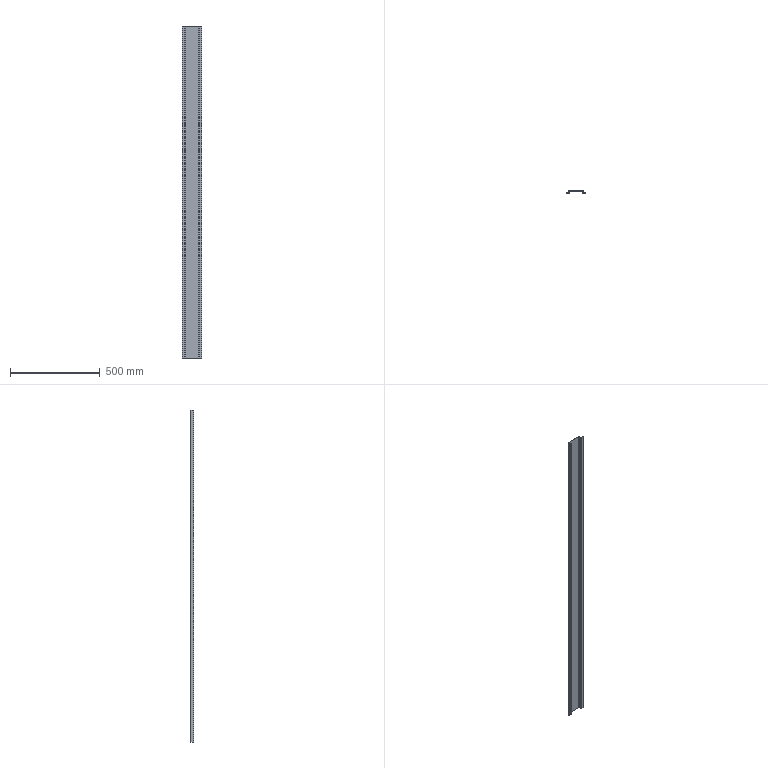Part | SolidWorks | features FlatPattern 1, SMBaseFlange 1, SheetMetal 1 | 1 solid | 38 faces | box 110 x 17 x 1845 mm | volume 384278 mm3 | plane 30 | cylinder 8 | commonest cylinder face diameters 1 x4 4 x4
STEP:
#1=CARTESIAN_POINT('',(-40.,0.5,922.5));
#2=VERTEX_POINT('',#1);
#3=CARTESIAN_POINT('',(-38.5,0.5,922.5));
#4=VERTEX_POINT('',#3);
#5=CARTESIAN_POINT('',(-40.,0.5,922.5));
#6=DIRECTION('',(1.,0.,0.));
#7=VECTOR('',#6,1000.);
#8=LINE('',#5,#7);
#9=EDGE_CURVE('',#2,#4,#8,.T.);
#10=ORIENTED_EDGE('',*,*,#9,.F.);
#11=CARTESIAN_POINT('',(-40.5,0.,922.5));
#12=VERTEX_POINT('',#11);
#13=CARTESIAN_POINT('',(-40.5,0.5,922.5));
#14=DIRECTION('',(0.,0.,-1.));
#15=DIRECTION('',(-1.,0.,0.));
#16=AXIS2_PLACEMENT_3D('',#13,#14,#15);
#17=CIRCLE('',#16,0.5);
#18=EDGE_CURVE('',#2,#12,#17,.T.);
#19=ORIENTED_EDGE('',*,*,#18,.T.);
#20=CARTESIAN_POINT('',(-40.5,-1.5,922.5));
#21=VERTEX_POINT('',#20);
#22=CARTESIAN_POINT('',(-40.5,-1.5,922.5));
#23=DIRECTION('',(0.,1.,0.));
#24=VECTOR('',#23,1000.);
#25=LINE('',#22,#24);
#26=EDGE_CURVE('',#21,#12,#25,.T.);
#27=ORIENTED_EDGE('',*,*,#26,.F.);
#28=CARTESIAN_POINT('',(-40.5,0.5,922.5));
#29=DIRECTION('',(0.,0.,-1.));
#30=DIRECTION('',(1.,0.,0.));
#31=AXIS2_PLACEMENT_3D('',#28,#29,#30);
#32=CIRCLE('',#31,2.);
#33=EDGE_CURVE('',#4,#21,#32,.T.);
#34=ORIENTED_EDGE('',*,*,#33,.F.);
#35=EDGE_LOOP('',(#10,#19,#27,#34));
#36=FACE_OUTER_BOUND('',#35,.T.);
#37=CARTESIAN_POINT('',(-40.,0.5,922.5));
#38=DIRECTION('',(0.,0.,1.));
#39=DIRECTION('',(1.,0.,0.));
#40=AXIS2_PLACEMENT_3D('',#37,#38,#39);
#41=PLANE('',#40);
#42=ADVANCED_FACE('',(#36),#41,.T.);
#43=CARTESIAN_POINT('',(-40.,13.5,922.5));
#44=VERTEX_POINT('',#43);
#45=CARTESIAN_POINT('',(-40.,0.,922.5));
#46=DIRECTION('',(0.,-1.,0.));
#47=VECTOR('',#46,1000.);
#48=LINE('',#45,#47);
#49=EDGE_CURVE('',#44,#2,#48,.T.);
#50=ORIENTED_EDGE('',*,*,#49,.T.);
#51=ORIENTED_EDGE('',*,*,#9,.T.);
#52=CARTESIAN_POINT('',(-38.5,13.5,922.5));
#53=VERTEX_POINT('',#52);
#54=CARTESIAN_POINT('',(-38.5,0.,922.5));
#55=DIRECTION('',(0.,-1.,0.));
#56=VECTOR('',#55,1000.);
#57=LINE('',#54,#56);
#58=EDGE_CURVE('',#53,#4,#57,.T.);
#59=ORIENTED_EDGE('',*,*,#58,.F.);
#60=CARTESIAN_POINT('',(-38.5,13.5,922.5));
#61=DIRECTION('',(-1.,0.,0.));
#62=VECTOR('',#61,1000.);
#63=LINE('',#60,#62);
#64=EDGE_CURVE('',#53,#44,#63,.T.);
#65=ORIENTED_EDGE('',*,*,#64,.T.);
#66=EDGE_LOOP('',(#50,#51,#59,#65));
#67=FACE_OUTER_BOUND('',#66,.T.);
#68=CARTESIAN_POINT('',(-40.5,-1.5,922.5));
#69=DIRECTION('',(0.,0.,1.));
#70=DIRECTION('',(1.,0.,0.));
#71=AXIS2_PLACEMENT_3D('',#68,#69,#70);
#72=PLANE('',#71);
#73=ADVANCED_FACE('',(#67),#72,.T.);
#74=CARTESIAN_POINT('',(-40.5,0.,-922.5));
#75=VERTEX_POINT('',#74);
#76=CARTESIAN_POINT('',(-40.5,-1.5,-922.5));
#77=VERTEX_POINT('',#76);
#78=CARTESIAN_POINT('',(-40.5,0.,-922.5));
#79=DIRECTION('',(0.,-1.,0.));
#80=VECTOR('',#79,1000.);
#81=LINE('',#78,#80);
#82=EDGE_CURVE('',#75,#77,#81,.T.);
#83=ORIENTED_EDGE('',*,*,#82,.F.);
#84=CARTESIAN_POINT('',(-40.,0.5,-922.5));
#85=VERTEX_POINT('',#84);
#86=CARTESIAN_POINT('',(-40.5,0.5,-922.5));
#87=DIRECTION('',(0.,0.,-1.));
#88=DIRECTION('',(-1.,0.,0.));
#89=AXIS2_PLACEMENT_3D('',#86,#87,#88);
#90=CIRCLE('',#89,0.5);
#91=EDGE_CURVE('',#85,#75,#90,.T.);
#92=ORIENTED_EDGE('',*,*,#91,.F.);
#93=CARTESIAN_POINT('',(-38.5,0.5,-922.5));
#94=VERTEX_POINT('',#93);
#95=CARTESIAN_POINT('',(-38.5,0.5,-922.5));
#96=DIRECTION('',(-1.,0.,0.));
#97=VECTOR('',#96,1000.);
#98=LINE('',#95,#97);
#99=EDGE_CURVE('',#94,#85,#98,.T.);
#100=ORIENTED_EDGE('',*,*,#99,.F.);
#101=CARTESIAN_POINT('',(-40.5,0.5,-922.5));
#102=DIRECTION('',(0.,0.,-1.));
#103=DIRECTION('',(1.,0.,0.));
#104=AXIS2_PLACEMENT_3D('',#101,#102,#103);
#105=CIRCLE('',#104,2.);
#106=EDGE_CURVE('',#94,#77,#105,.T.);
#107=ORIENTED_EDGE('',*,*,#106,.T.);
#108=EDGE_LOOP('',(#83,#92,#100,#107));
#109=FACE_OUTER_BOUND('',#108,.T.);
#110=CARTESIAN_POINT('',(-40.5,0.,-922.5));
#111=DIRECTION('',(0.,0.,-1.));
#112=DIRECTION('',(-1.,0.,0.));
#113=AXIS2_PLACEMENT_3D('',#110,#111,#112);
#114=PLANE('',#113);
#115=ADVANCED_FACE('',(#109),#114,.T.);
#116=CARTESIAN_POINT('',(-55.,0.,-922.5));
#117=VERTEX_POINT('',#116);
#118=CARTESIAN_POINT('',(-55.,0.,-922.5));
#119=DIRECTION('',(-1.,0.,0.));
#120=VECTOR('',#119,1000.);
#121=LINE('',#118,#120);
#122=EDGE_CURVE('',#75,#117,#121,.T.);
#123=ORIENTED_EDGE('',*,*,#122,.F.);
#124=ORIENTED_EDGE('',*,*,#82,.T.);
#125=CARTESIAN_POINT('',(-55.,-1.5,-922.5));
#126=VERTEX_POINT('',#125);
#127=CARTESIAN_POINT('',(-55.,-1.5,-922.5));
#128=DIRECTION('',(-1.,0.,0.));
#129=VECTOR('',#128,1000.);
#130=LINE('',#127,#129);
#131=EDGE_CURVE('',#77,#126,#130,.T.);
#132=ORIENTED_EDGE('',*,*,#131,.T.);
#133=CARTESIAN_POINT('',(-55.,-1.5,-922.5));
#134=DIRECTION('',(0.,1.,0.));
#135=VECTOR('',#134,1000.);
#136=LINE('',#133,#135);
#137=EDGE_CURVE('',#126,#117,#136,.T.);
#138=ORIENTED_EDGE('',*,*,#137,.T.);
#139=EDGE_LOOP('',(#123,#124,#132,#138));
#140=FACE_OUTER_BOUND('',#139,.T.);
#141=CARTESIAN_POINT('',(-38.5,0.5,-922.5));
#142=DIRECTION('',(0.,0.,-1.));
#143=DIRECTION('',(-1.,0.,0.));
#144=AXIS2_PLACEMENT_3D('',#141,#142,#143);
#145=PLANE('',#144);
#146=ADVANCED_FACE('',(#140),#145,.T.);
#147=CARTESIAN_POINT('',(-38.,15.5,922.5));
#148=VERTEX_POINT('',#147);
#149=CARTESIAN_POINT('',(-38.,14.,922.5));
#150=VERTEX_POINT('',#149);
#151=CARTESIAN_POINT('',(-38.,15.5,922.5));
#152=DIRECTION('',(0.,-1.,0.));
#153=VECTOR('',#152,1000.);
#154=LINE('',#151,#153);
#155=EDGE_CURVE('',#148,#150,#154,.T.);
#156=ORIENTED_EDGE('',*,*,#155,.F.);
#157=CARTESIAN_POINT('',(-38.,13.5,922.5));
#158=DIRECTION('',(0.,0.,1.));
#159=DIRECTION('',(1.,0.,0.));
#160=AXIS2_PLACEMENT_3D('',#157,#158,#159);
#161=CIRCLE('',#160,2.);
#162=EDGE_CURVE('',#148,#44,#161,.T.);
#163=ORIENTED_EDGE('',*,*,#162,.T.);
#164=ORIENTED_EDGE('',*,*,#64,.F.);
#165=CARTESIAN_POINT('',(-38.,13.5,922.5));
#166=DIRECTION('',(0.,0.,1.));
#167=DIRECTION('',(1.,0.,0.));
#168=AXIS2_PLACEMENT_3D('',#165,#166,#167);
#169=CIRCLE('',#168,0.5);
#170=EDGE_CURVE('',#150,#53,#169,.T.);
#171=ORIENTED_EDGE('',*,*,#170,.F.);
#172=EDGE_LOOP('',(#156,#163,#164,#171));
#173=FACE_OUTER_BOUND('',#172,.T.);
#174=CARTESIAN_POINT('',(-38.,15.5,922.5));
#175=DIRECTION('',(0.,0.,1.));
#176=DIRECTION('',(1.,0.,0.));
#177=AXIS2_PLACEMENT_3D('',#174,#175,#176);
#178=PLANE('',#177);
#179=ADVANCED_FACE('',(#173),#178,.T.);
#180=CARTESIAN_POINT('',(38.,15.5,922.5));
#181=VERTEX_POINT('',#180);
#182=CARTESIAN_POINT('',(-40.,15.5,922.5));
#183=DIRECTION('',(-1.,0.,0.));
#184=VECTOR('',#183,1000.);
#185=LINE('',#182,#184);
#186=EDGE_CURVE('',#181,#148,#185,.T.);
#187=ORIENTED_EDGE('',*,*,#186,.T.);
#188=ORIENTED_EDGE('',*,*,#155,.T.);
#189=CARTESIAN_POINT('',(38.,14.,922.5));
#190=VERTEX_POINT('',#189);
#191=CARTESIAN_POINT('',(-40.,14.,922.5));
#192=DIRECTION('',(-1.,0.,0.));
#193=VECTOR('',#192,1000.);
#194=LINE('',#191,#193);
#195=EDGE_CURVE('',#190,#150,#194,.T.);
#196=ORIENTED_EDGE('',*,*,#195,.F.);
#197=CARTESIAN_POINT('',(38.,14.,922.5));
#198=DIRECTION('',(0.,1.,0.));
#199=VECTOR('',#198,1000.);
#200=LINE('',#197,#199);
#201=EDGE_CURVE('',#190,#181,#200,.T.);
#202=ORIENTED_EDGE('',*,*,#201,.T.);
#203=EDGE_LOOP('',(#187,#188,#196,#202));
#204=FACE_OUTER_BOUND('',#203,.T.);
#205=CARTESIAN_POINT('',(-38.5,13.5,922.5));
#206=DIRECTION('',(0.,0.,1.));
#207=DIRECTION('',(1.,0.,0.));
#208=AXIS2_PLACEMENT_3D('',#205,#206,#207);
#209=PLANE('',#208);
#210=ADVANCED_FACE('',(#204),#209,.T.);
#211=CARTESIAN_POINT('',(-40.,13.5,-922.5));
#212=VERTEX_POINT('',#211);
#213=CARTESIAN_POINT('',(-38.5,13.5,-922.5));
#214=VERTEX_POINT('',#213);
#215=CARTESIAN_POINT('',(-40.,13.5,-922.5));
#216=DIRECTION('',(1.,0.,0.));
#217=VECTOR('',#216,1000.);
#218=LINE('',#215,#217);
#219=EDGE_CURVE('',#212,#214,#218,.T.);
#220=ORIENTED_EDGE('',*,*,#219,.F.);
#221=CARTESIAN_POINT('',(-38.,15.5,-922.5));
#222=VERTEX_POINT('',#221);
#223=CARTESIAN_POINT('',(-38.,13.5,-922.5));
#224=DIRECTION('',(0.,0.,1.));
#225=DIRECTION('',(1.,0.,0.));
#226=AXIS2_PLACEMENT_3D('',#223,#224,#225);
#227=CIRCLE('',#226,2.);
#228=EDGE_CURVE('',#222,#212,#227,.T.);
#229=ORIENTED_EDGE('',*,*,#228,.F.);
#230=CARTESIAN_POINT('',(-38.,14.,-922.5));
#231=VERTEX_POINT('',#230);
#232=CARTESIAN_POINT('',(-38.,14.,-922.5));
#233=DIRECTION('',(0.,1.,0.));
#234=VECTOR('',#233,1000.);
#235=LINE('',#232,#234);
#236=EDGE_CURVE('',#231,#222,#235,.T.);
#237=ORIENTED_EDGE('',*,*,#236,.F.);
#238=CARTESIAN_POINT('',(-38.,13.5,-922.5));
#239=DIRECTION('',(0.,0.,1.));
#240=DIRECTION('',(1.,0.,0.));
#241=AXIS2_PLACEMENT_3D('',#238,#239,#240);
#242=CIRCLE('',#241,0.5);
#243=EDGE_CURVE('',#231,#214,#242,.T.);
#244=ORIENTED_EDGE('',*,*,#243,.T.);
#245=EDGE_LOOP('',(#220,#229,#237,#244));
#246=FACE_OUTER_BOUND('',#245,.T.);
#247=CARTESIAN_POINT('',(-40.,13.5,-922.5));
#248=DIRECTION('',(0.,0.,-1.));
#249=DIRECTION('',(-1.,0.,0.));
#250=AXIS2_PLACEMENT_3D('',#247,#248,#249);
#251=PLANE('',#250);
#252=ADVANCED_FACE('',(#246),#251,.T.);
#253=CARTESIAN_POINT('',(-40.,0.,-922.5));
#254=DIRECTION('',(0.,-1.,0.));
#255=VECTOR('',#254,1000.);
#256=LINE('',#253,#255);
#257=EDGE_CURVE('',#212,#85,#256,.T.);
#258=ORIENTED_EDGE('',*,*,#257,.F.);
#259=ORIENTED_EDGE('',*,*,#219,.T.);
#260=CARTESIAN_POINT('',(-38.5,0.,-922.5));
#261=DIRECTION('',(0.,-1.,0.));
#262=VECTOR('',#261,1000.);
#263=LINE('',#260,#262);
#264=EDGE_CURVE('',#214,#94,#263,.T.);
#265=ORIENTED_EDGE('',*,*,#264,.T.);
#266=ORIENTED_EDGE('',*,*,#99,.T.);
#267=EDGE_LOOP('',(#258,#259,#265,#266));
#268=FACE_OUTER_BOUND('',#267,.T.);
#269=CARTESIAN_POINT('',(-38.,14.,-922.5));
#270=DIRECTION('',(0.,0.,-1.));
#271=DIRECTION('',(-1.,0.,0.));
#272=AXIS2_PLACEMENT_3D('',#269,#270,#271);
#273=PLANE('',#272);
#274=ADVANCED_FACE('',(#268),#273,.T.);
#275=CARTESIAN_POINT('',(40.,13.5,922.5));
#276=VERTEX_POINT('',#275);
#277=CARTESIAN_POINT('',(38.5,13.5,922.5));
#278=VERTEX_POINT('',#277);
#279=CARTESIAN_POINT('',(40.,13.5,922.5));
#280=DIRECTION('',(-1.,0.,0.));
#281=VECTOR('',#280,1000.);
#282=LINE('',#279,#281);
#283=EDGE_CURVE('',#276,#278,#282,.T.);
#284=ORIENTED_EDGE('',*,*,#283,.F.);
#285=CARTESIAN_POINT('',(38.,13.5,922.5));
#286=DIRECTION('',(0.,0.,1.));
#287=DIRECTION('',(1.,0.,0.));
#288=AXIS2_PLACEMENT_3D('',#285,#286,#287);
#289=CIRCLE('',#288,2.);
#290=EDGE_CURVE('',#276,#181,#289,.T.);
#291=ORIENTED_EDGE('',*,*,#290,.T.);
#292=ORIENTED_EDGE('',*,*,#201,.F.);
#293=CARTESIAN_POINT('',(38.,13.5,922.5));
#294=DIRECTION('',(0.,0.,1.));
#295=DIRECTION('',(1.,0.,0.));
#296=AXIS2_PLACEMENT_3D('',#293,#294,#295);
#297=CIRCLE('',#296,0.5);
#298=EDGE_CURVE('',#278,#190,#297,.T.);
#299=ORIENTED_EDGE('',*,*,#298,.F.);
#300=EDGE_LOOP('',(#284,#291,#292,#299));
#301=FACE_OUTER_BOUND('',#300,.T.);
#302=CARTESIAN_POINT('',(40.,13.5,922.5));
#303=DIRECTION('',(0.,0.,1.));
#304=DIRECTION('',(1.,0.,0.));
#305=AXIS2_PLACEMENT_3D('',#302,#303,#304);
#306=PLANE('',#305);
#307=ADVANCED_FACE('',(#301),#306,.T.);
#308=CARTESIAN_POINT('',(40.,0.5,922.5));
#309=VERTEX_POINT('',#308);
#310=CARTESIAN_POINT('',(40.,0.,922.5));
#311=DIRECTION('',(0.,1.,0.));
#312=VECTOR('',#311,1000.);
#313=LINE('',#310,#312);
#314=EDGE_CURVE('',#309,#276,#313,.T.);
#315=ORIENTED_EDGE('',*,*,#314,.T.);
#316=ORIENTED_EDGE('',*,*,#283,.T.);
#317=CARTESIAN_POINT('',(38.5,0.5,922.5));
#318=VERTEX_POINT('',#317);
#319=CARTESIAN_POINT('',(38.5,0.,922.5));
#320=DIRECTION('',(0.,1.,0.));
#321=VECTOR('',#320,1000.);
#322=LINE('',#319,#321);
#323=EDGE_CURVE('',#318,#278,#322,.T.);
#324=ORIENTED_EDGE('',*,*,#323,.F.);
#325=CARTESIAN_POINT('',(38.5,0.5,922.5));
#326=DIRECTION('',(1.,0.,0.));
#327=VECTOR('',#326,1000.);
#328=LINE('',#325,#327);
#329=EDGE_CURVE('',#318,#309,#328,.T.);
#330=ORIENTED_EDGE('',*,*,#329,.T.);
#331=EDGE_LOOP('',(#315,#316,#324,#330));
#332=FACE_OUTER_BOUND('',#331,.T.);
#333=CARTESIAN_POINT('',(38.,14.,922.5));
#334=DIRECTION('',(0.,0.,1.));
#335=DIRECTION('',(1.,0.,0.));
#336=AXIS2_PLACEMENT_3D('',#333,#334,#335);
#337=PLANE('',#336);
#338=ADVANCED_FACE('',(#332),#337,.T.);
#339=CARTESIAN_POINT('',(38.,15.5,-922.5));
#340=VERTEX_POINT('',#339);
#341=CARTESIAN_POINT('',(38.,14.,-922.5));
#342=VERTEX_POINT('',#341);
#343=CARTESIAN_POINT('',(38.,15.5,-922.5));
#344=DIRECTION('',(0.,-1.,0.));
#345=VECTOR('',#344,1000.);
#346=LINE('',#343,#345);
#347=EDGE_CURVE('',#340,#342,#346,.T.);
#348=ORIENTED_EDGE('',*,*,#347,.F.);
#349=CARTESIAN_POINT('',(40.,13.5,-922.5));
#350=VERTEX_POINT('',#349);
#351=CARTESIAN_POINT('',(38.,13.5,-922.5));
#352=DIRECTION('',(0.,0.,1.));
#353=DIRECTION('',(1.,0.,0.));
#354=AXIS2_PLACEMENT_3D('',#351,#352,#353);
#355=CIRCLE('',#354,2.);
#356=EDGE_CURVE('',#350,#340,#355,.T.);
#357=ORIENTED_EDGE('',*,*,#356,.F.);
#358=CARTESIAN_POINT('',(38.5,13.5,-922.5));
#359=VERTEX_POINT('',#358);
#360=CARTESIAN_POINT('',(38.5,13.5,-922.5));
#361=DIRECTION('',(1.,0.,0.));
#362=VECTOR('',#361,1000.);
#363=LINE('',#360,#362);
#364=EDGE_CURVE('',#359,#350,#363,.T.);
#365=ORIENTED_EDGE('',*,*,#364,.F.);
#366=CARTESIAN_POINT('',(38.,13.5,-922.5));
#367=DIRECTION('',(0.,0.,1.));
#368=DIRECTION('',(1.,0.,0.));
#369=AXIS2_PLACEMENT_3D('',#366,#367,#368);
#370=CIRCLE('',#369,0.5);
#371=EDGE_CURVE('',#359,#342,#370,.T.);
#372=ORIENTED_EDGE('',*,*,#371,.T.);
#373=EDGE_LOOP('',(#348,#357,#365,#372));
#374=FACE_OUTER_BOUND('',#373,.T.);
#375=CARTESIAN_POINT('',(38.,15.5,-922.5));
#376=DIRECTION('',(0.,0.,-1.));
#377=DIRECTION('',(-1.,0.,0.));
#378=AXIS2_PLACEMENT_3D('',#375,#376,#377);
#379=PLANE('',#378);
#380=ADVANCED_FACE('',(#374),#379,.T.);
#381=CARTESIAN_POINT('',(-40.,15.5,-922.5));
#382=DIRECTION('',(-1.,0.,0.));
#383=VECTOR('',#382,1000.);
#384=LINE('',#381,#383);
#385=EDGE_CURVE('',#340,#222,#384,.T.);
#386=ORIENTED_EDGE('',*,*,#385,.F.);
#387=ORIENTED_EDGE('',*,*,#347,.T.);
#388=CARTESIAN_POINT('',(-40.,14.,-922.5));
#389=DIRECTION('',(-1.,0.,0.));
#390=VECTOR('',#389,1000.);
#391=LINE('',#388,#390);
#392=EDGE_CURVE('',#342,#231,#391,.T.);
#393=ORIENTED_EDGE('',*,*,#392,.T.);
#394=ORIENTED_EDGE('',*,*,#236,.T.);
#395=EDGE_LOOP('',(#386,#387,#393,#394));
#396=FACE_OUTER_BOUND('',#395,.T.);
#397=CARTESIAN_POINT('',(38.5,13.5,-922.5));
#398=DIRECTION('',(0.,0.,-1.));
#399=DIRECTION('',(-1.,0.,0.));
#400=AXIS2_PLACEMENT_3D('',#397,#398,#399);
#401=PLANE('',#400);
#402=ADVANCED_FACE('',(#396),#401,.T.);
#403=CARTESIAN_POINT('',(40.5,0.,922.5));
#404=VERTEX_POINT('',#403);
#405=CARTESIAN_POINT('',(40.5,-1.5,922.5));
#406=VERTEX_POINT('',#405);
#407=CARTESIAN_POINT('',(40.5,0.,922.5));
#408=DIRECTION('',(0.,-1.,0.));
#409=VECTOR('',#408,1000.);
#410=LINE('',#407,#409);
#411=EDGE_CURVE('',#404,#406,#410,.T.);
#412=ORIENTED_EDGE('',*,*,#411,.F.);
#413=CARTESIAN_POINT('',(40.5,0.5,922.5));
#414=DIRECTION('',(0.,0.,-1.));
#415=DIRECTION('',(-1.,0.,0.));
#416=AXIS2_PLACEMENT_3D('',#413,#414,#415);
#417=CIRCLE('',#416,0.5);
#418=EDGE_CURVE('',#404,#309,#417,.T.);
#419=ORIENTED_EDGE('',*,*,#418,.T.);
#420=ORIENTED_EDGE('',*,*,#329,.F.);
#421=CARTESIAN_POINT('',(40.5,0.5,922.5));
#422=DIRECTION('',(0.,0.,-1.));
#423=DIRECTION('',(1.,0.,0.));
#424=AXIS2_PLACEMENT_3D('',#421,#422,#423);
#425=CIRCLE('',#424,2.);
#426=EDGE_CURVE('',#406,#318,#425,.T.);
#427=ORIENTED_EDGE('',*,*,#426,.F.);
#428=EDGE_LOOP('',(#412,#419,#420,#427));
#429=FACE_OUTER_BOUND('',#428,.T.);
#430=CARTESIAN_POINT('',(40.5,0.,922.5));
#431=DIRECTION('',(0.,0.,1.));
#432=DIRECTION('',(1.,0.,0.));
#433=AXIS2_PLACEMENT_3D('',#430,#431,#432);
#434=PLANE('',#433);
#435=ADVANCED_FACE('',(#429),#434,.T.);
#436=CARTESIAN_POINT('',(55.,0.,922.5));
#437=VERTEX_POINT('',#436);
#438=CARTESIAN_POINT('',(55.,0.,922.5));
#439=DIRECTION('',(-1.,0.,0.));
#440=VECTOR('',#439,1000.);
#441=LINE('',#438,#440);
#442=EDGE_CURVE('',#437,#404,#441,.T.);
#443=ORIENTED_EDGE('',*,*,#442,.T.);
#444=ORIENTED_EDGE('',*,*,#411,.T.);
#445=CARTESIAN_POINT('',(55.,-1.5,922.5));
#446=VERTEX_POINT('',#445);
#447=CARTESIAN_POINT('',(55.,-1.5,922.5));
#448=DIRECTION('',(-1.,0.,0.));
#449=VECTOR('',#448,1000.);
#450=LINE('',#447,#449);
#451=EDGE_CURVE('',#446,#406,#450,.T.);
#452=ORIENTED_EDGE('',*,*,#451,.F.);
#453=CARTESIAN_POINT('',(55.,0.,922.5));
#454=DIRECTION('',(0.,-1.,0.));
#455=VECTOR('',#454,1000.);
#456=LINE('',#453,#455);
#457=EDGE_CURVE('',#437,#446,#456,.T.);
#458=ORIENTED_EDGE('',*,*,#457,.F.);
#459=EDGE_LOOP('',(#443,#444,#452,#458));
#460=FACE_OUTER_BOUND('',#459,.T.);
#461=CARTESIAN_POINT('',(38.5,0.5,922.5));
#462=DIRECTION('',(0.,0.,1.));
#463=DIRECTION('',(1.,0.,0.));
#464=AXIS2_PLACEMENT_3D('',#461,#462,#463);
#465=PLANE('',#464);
#466=ADVANCED_FACE('',(#460),#465,.T.);
#467=CARTESIAN_POINT('',(40.,0.5,-922.5));
#468=VERTEX_POINT('',#467);
#469=CARTESIAN_POINT('',(38.5,0.5,-922.5));
#470=VERTEX_POINT('',#469);
#471=CARTESIAN_POINT('',(40.,0.5,-922.5));
#472=DIRECTION('',(-1.,0.,0.));
#473=VECTOR('',#472,1000.);
#474=LINE('',#471,#473);
#475=EDGE_CURVE('',#468,#470,#474,.T.);
#476=ORIENTED_EDGE('',*,*,#475,.F.);
#477=CARTESIAN_POINT('',(40.5,0.,-922.5));
#478=VERTEX_POINT('',#477);
#479=CARTESIAN_POINT('',(40.5,0.5,-922.5));
#480=DIRECTION('',(0.,0.,-1.));
#481=DIRECTION('',(-1.,0.,0.));
#482=AXIS2_PLACEMENT_3D('',#479,#480,#481);
#483=CIRCLE('',#482,0.5);
#484=EDGE_CURVE('',#478,#468,#483,.T.);
#485=ORIENTED_EDGE('',*,*,#484,.F.);
#486=CARTESIAN_POINT('',(40.5,-1.5,-922.5));
#487=VERTEX_POINT('',#486);
#488=CARTESIAN_POINT('',(40.5,-1.5,-922.5));
#489=DIRECTION('',(0.,1.,0.));
#490=VECTOR('',#489,1000.);
#491=LINE('',#488,#490);
#492=EDGE_CURVE('',#487,#478,#491,.T.);
#493=ORIENTED_EDGE('',*,*,#492,.F.);
#494=CARTESIAN_POINT('',(40.5,0.5,-922.5));
#495=DIRECTION('',(0.,0.,-1.));
#496=DIRECTION('',(1.,0.,0.));
#497=AXIS2_PLACEMENT_3D('',#494,#495,#496);
#498=CIRCLE('',#497,2.);
#499=EDGE_CURVE('',#487,#470,#498,.T.);
#500=ORIENTED_EDGE('',*,*,#499,.T.);
#501=EDGE_LOOP('',(#476,#485,#493,#500));
#502=FACE_OUTER_BOUND('',#501,.T.);
#503=CARTESIAN_POINT('',(40.,0.5,-922.5));
#504=DIRECTION('',(0.,0.,-1.));
#505=DIRECTION('',(-1.,0.,0.));
#506=AXIS2_PLACEMENT_3D('',#503,#504,#505);
#507=PLANE('',#506);
#508=ADVANCED_FACE('',(#502),#507,.T.);
#509=CARTESIAN_POINT('',(40.,0.,-922.5));
#510=DIRECTION('',(0.,1.,0.));
#511=VECTOR('',#510,1000.);
#512=LINE('',#509,#511);
#513=EDGE_CURVE('',#468,#350,#512,.T.);
#514=ORIENTED_EDGE('',*,*,#513,.F.);
#515=ORIENTED_EDGE('',*,*,#475,.T.);
#516=CARTESIAN_POINT('',(38.5,0.,-922.5));
#517=DIRECTION('',(0.,1.,0.));
#518=VECTOR('',#517,1000.);
#519=LINE('',#516,#518);
#520=EDGE_CURVE('',#470,#359,#519,.T.);
#521=ORIENTED_EDGE('',*,*,#520,.T.);
#522=ORIENTED_EDGE('',*,*,#364,.T.);
#523=EDGE_LOOP('',(#514,#515,#521,#522));
#524=FACE_OUTER_BOUND('',#523,.T.);
#525=CARTESIAN_POINT('',(40.5,-1.5,-922.5));
#526=DIRECTION('',(0.,0.,-1.));
#527=DIRECTION('',(-1.,0.,0.));
#528=AXIS2_PLACEMENT_3D('',#525,#526,#527);
#529=PLANE('',#528);
#530=ADVANCED_FACE('',(#524),#529,.T.);
#531=ORIENTED_EDGE('',*,*,#122,.T.);
#532=CARTESIAN_POINT('',(-55.,0.,922.5));
#533=VERTEX_POINT('',#532);
#534=CARTESIAN_POINT('',(-55.,0.,922.5));
#535=DIRECTION('',(0.,0.,-1.));
#536=VECTOR('',#535,1000.);
#537=LINE('',#534,#536);
#538=EDGE_CURVE('',#533,#117,#537,.T.);
#539=ORIENTED_EDGE('',*,*,#538,.F.);
#540=CARTESIAN_POINT('',(-55.,0.,922.5));
#541=DIRECTION('',(-1.,0.,0.));
#542=VECTOR('',#541,1000.);
#543=LINE('',#540,#542);
#544=EDGE_CURVE('',#12,#533,#543,.T.);
#545=ORIENTED_EDGE('',*,*,#544,.F.);
#546=CARTESIAN_POINT('',(-40.5,0.,922.5));
#547=DIRECTION('',(0.,0.,-1.));
#548=VECTOR('',#547,1000.);
#549=LINE('',#546,#548);
#550=EDGE_CURVE('',#12,#75,#549,.T.);
#551=ORIENTED_EDGE('',*,*,#550,.T.);
#552=EDGE_LOOP('',(#531,#539,#545,#551));
#553=FACE_OUTER_BOUND('',#552,.T.);
#554=CARTESIAN_POINT('',(-55.,0.,922.5));
#555=DIRECTION('',(0.,-1.,0.));
#556=DIRECTION('',(0.,0.,-1.));
#557=AXIS2_PLACEMENT_3D('',#554,#555,#556);
#558=PLANE('',#557);
#559=ADVANCED_FACE('',(#553),#558,.F.);
#560=ORIENTED_EDGE('',*,*,#137,.F.);
#561=CARTESIAN_POINT('',(-55.,-1.5,922.5));
#562=VERTEX_POINT('',#561);
#563=CARTESIAN_POINT('',(-55.,-1.5,922.5));
#564=DIRECTION('',(0.,0.,-1.));
#565=VECTOR('',#564,1000.);
#566=LINE('',#563,#565);
#567=EDGE_CURVE('',#562,#126,#566,.T.);
#568=ORIENTED_EDGE('',*,*,#567,.F.);
#569=CARTESIAN_POINT('',(-55.,-1.5,922.5));
#570=DIRECTION('',(0.,1.,0.));
#571=VECTOR('',#570,1000.);
#572=LINE('',#569,#571);
#573=EDGE_CURVE('',#562,#533,#572,.T.);
#574=ORIENTED_EDGE('',*,*,#573,.T.);
#575=ORIENTED_EDGE('',*,*,#538,.T.);
#576=EDGE_LOOP('',(#560,#568,#574,#575));
#577=FACE_OUTER_BOUND('',#576,.T.);
#578=CARTESIAN_POINT('',(-55.,-1.5,922.5));
#579=DIRECTION('',(-1.,0.,0.));
#580=DIRECTION('',(0.,0.,1.));
#581=AXIS2_PLACEMENT_3D('',#578,#579,#580);
#582=PLANE('',#581);
#583=ADVANCED_FACE('',(#577),#582,.T.);
#584=ORIENTED_EDGE('',*,*,#131,.F.);
#585=CARTESIAN_POINT('',(-40.5,-1.5,922.5));
#586=DIRECTION('',(0.,0.,-1.));
#587=VECTOR('',#586,1000.);
#588=LINE('',#585,#587);
#589=EDGE_CURVE('',#21,#77,#588,.T.);
#590=ORIENTED_EDGE('',*,*,#589,.F.);
#591=CARTESIAN_POINT('',(-55.,-1.5,922.5));
#592=DIRECTION('',(-1.,0.,0.));
#593=VECTOR('',#592,1000.);
#594=LINE('',#591,#593);
#595=EDGE_CURVE('',#21,#562,#594,.T.);
#596=ORIENTED_EDGE('',*,*,#595,.T.);
#597=ORIENTED_EDGE('',*,*,#567,.T.);
#598=EDGE_LOOP('',(#584,#590,#596,#597));
#599=FACE_OUTER_BOUND('',#598,.T.);
#600=CARTESIAN_POINT('',(-55.,-1.5,922.5));
#601=DIRECTION('',(0.,-1.,0.));
#602=DIRECTION('',(0.,0.,-1.));
#603=AXIS2_PLACEMENT_3D('',#600,#601,#602);
#604=PLANE('',#603);
#605=ADVANCED_FACE('',(#599),#604,.T.);
#606=ORIENTED_EDGE('',*,*,#106,.F.);
#607=CARTESIAN_POINT('',(-38.5,0.5,922.5));
#608=DIRECTION('',(0.,0.,-1.));
#609=VECTOR('',#608,1000.);
#610=LINE('',#607,#609);
#611=EDGE_CURVE('',#4,#94,#610,.T.);
#612=ORIENTED_EDGE('',*,*,#611,.F.);
#613=ORIENTED_EDGE('',*,*,#33,.T.);
#614=ORIENTED_EDGE('',*,*,#589,.T.);
#615=EDGE_LOOP('',(#606,#612,#613,#614));
#616=FACE_OUTER_BOUND('',#615,.T.);
#617=CARTESIAN_POINT('',(-40.5,0.5,922.5));
#618=DIRECTION('',(0.,0.,-1.));
#619=DIRECTION('',(-1.,0.,0.));
#620=AXIS2_PLACEMENT_3D('',#617,#618,#619);
#621=CYLINDRICAL_SURFACE('',#620,2.);
#622=ADVANCED_FACE('',(#616),#621,.T.);
#623=ORIENTED_EDGE('',*,*,#264,.F.);
#624=CARTESIAN_POINT('',(-38.5,13.5,922.5));
#625=DIRECTION('',(0.,0.,-1.));
#626=VECTOR('',#625,1000.);
#627=LINE('',#624,#626);
#628=EDGE_CURVE('',#53,#214,#627,.T.);
#629=ORIENTED_EDGE('',*,*,#628,.F.);
#630=ORIENTED_EDGE('',*,*,#58,.T.);
#631=ORIENTED_EDGE('',*,*,#611,.T.);
#632=EDGE_LOOP('',(#623,#629,#630,#631));
#633=FACE_OUTER_BOUND('',#632,.T.);
#634=CARTESIAN_POINT('',(-38.5,0.,922.5));
#635=DIRECTION('',(1.,0.,0.));
#636=DIRECTION('',(0.,1.,0.));
#637=AXIS2_PLACEMENT_3D('',#634,#635,#636);
#638=PLANE('',#637);
#639=ADVANCED_FACE('',(#633),#638,.T.);
#640=ORIENTED_EDGE('',*,*,#243,.F.);
#641=CARTESIAN_POINT('',(-38.,14.,922.5));
#642=DIRECTION('',(0.,0.,-1.));
#643=VECTOR('',#642,1000.);
#644=LINE('',#641,#643);
#645=EDGE_CURVE('',#150,#231,#644,.T.);
#646=ORIENTED_EDGE('',*,*,#645,.F.);
#647=ORIENTED_EDGE('',*,*,#170,.T.);
#648=ORIENTED_EDGE('',*,*,#628,.T.);
#649=EDGE_LOOP('',(#640,#646,#647,#648));
#650=FACE_OUTER_BOUND('',#649,.T.);
#651=CARTESIAN_POINT('',(-38.,13.5,922.5));
#652=DIRECTION('',(0.,0.,-1.));
#653=DIRECTION('',(-1.,0.,0.));
#654=AXIS2_PLACEMENT_3D('',#651,#652,#653);
#655=CYLINDRICAL_SURFACE('',#654,0.5);
#656=ADVANCED_FACE('',(#650),#655,.F.);
#657=ORIENTED_EDGE('',*,*,#392,.F.);
#658=CARTESIAN_POINT('',(38.,14.,922.5));
#659=DIRECTION('',(0.,0.,-1.));
#660=VECTOR('',#659,1000.);
#661=LINE('',#658,#660);
#662=EDGE_CURVE('',#190,#342,#661,.T.);
#663=ORIENTED_EDGE('',*,*,#662,.F.);
#664=ORIENTED_EDGE('',*,*,#195,.T.);
#665=ORIENTED_EDGE('',*,*,#645,.T.);
#666=EDGE_LOOP('',(#657,#663,#664,#665));
#667=FACE_OUTER_BOUND('',#666,.T.);
#668=CARTESIAN_POINT('',(-40.,14.,922.5));
#669=DIRECTION('',(0.,-1.,0.));
#670=DIRECTION('',(0.,0.,-1.));
#671=AXIS2_PLACEMENT_3D('',#668,#669,#670);
#672=PLANE('',#671);
#673=ADVANCED_FACE('',(#667),#672,.T.);
#674=ORIENTED_EDGE('',*,*,#371,.F.);
#675=CARTESIAN_POINT('',(38.5,13.5,922.5));
#676=DIRECTION('',(0.,0.,-1.));
#677=VECTOR('',#676,1000.);
#678=LINE('',#675,#677);
#679=EDGE_CURVE('',#278,#359,#678,.T.);
#680=ORIENTED_EDGE('',*,*,#679,.F.);
#681=ORIENTED_EDGE('',*,*,#298,.T.);
#682=ORIENTED_EDGE('',*,*,#662,.T.);
#683=EDGE_LOOP('',(#674,#680,#681,#682));
#684=FACE_OUTER_BOUND('',#683,.T.);
#685=CARTESIAN_POINT('',(38.,13.5,922.5));
#686=DIRECTION('',(0.,0.,-1.));
#687=DIRECTION('',(-1.,0.,0.));
#688=AXIS2_PLACEMENT_3D('',#685,#686,#687);
#689=CYLINDRICAL_SURFACE('',#688,0.5);
#690=ADVANCED_FACE('',(#684),#689,.F.);
#691=ORIENTED_EDGE('',*,*,#520,.F.);
#692=CARTESIAN_POINT('',(38.5,0.5,922.5));
#693=DIRECTION('',(0.,0.,-1.));
#694=VECTOR('',#693,1000.);
#695=LINE('',#692,#694);
#696=EDGE_CURVE('',#318,#470,#695,.T.);
#697=ORIENTED_EDGE('',*,*,#696,.F.);
#698=ORIENTED_EDGE('',*,*,#323,.T.);
#699=ORIENTED_EDGE('',*,*,#679,.T.);
#700=EDGE_LOOP('',(#691,#697,#698,#699));
#701=FACE_OUTER_BOUND('',#700,.T.);
#702=CARTESIAN_POINT('',(38.5,0.,922.5));
#703=DIRECTION('',(-1.,0.,0.));
#704=DIRECTION('',(0.,-1.,0.));
#705=AXIS2_PLACEMENT_3D('',#702,#703,#704);
#706=PLANE('',#705);
#707=ADVANCED_FACE('',(#701),#706,.T.);
#708=ORIENTED_EDGE('',*,*,#499,.F.);
#709=CARTESIAN_POINT('',(40.5,-1.5,922.5));
#710=DIRECTION('',(0.,0.,-1.));
#711=VECTOR('',#710,1000.);
#712=LINE('',#709,#711);
#713=EDGE_CURVE('',#406,#487,#712,.T.);
#714=ORIENTED_EDGE('',*,*,#713,.F.);
#715=ORIENTED_EDGE('',*,*,#426,.T.);
#716=ORIENTED_EDGE('',*,*,#696,.T.);
#717=EDGE_LOOP('',(#708,#714,#715,#716));
#718=FACE_OUTER_BOUND('',#717,.T.);
#719=CARTESIAN_POINT('',(40.5,0.5,922.5));
#720=DIRECTION('',(0.,0.,-1.));
#721=DIRECTION('',(-1.,0.,0.));
#722=AXIS2_PLACEMENT_3D('',#719,#720,#721);
#723=CYLINDRICAL_SURFACE('',#722,2.);
#724=ADVANCED_FACE('',(#718),#723,.T.);
#725=CARTESIAN_POINT('',(55.,-1.5,-922.5));
#726=VERTEX_POINT('',#725);
#727=CARTESIAN_POINT('',(55.,-1.5,-922.5));
#728=DIRECTION('',(-1.,0.,0.));
#729=VECTOR('',#728,1000.);
#730=LINE('',#727,#729);
#731=EDGE_CURVE('',#726,#487,#730,.T.);
#732=ORIENTED_EDGE('',*,*,#731,.F.);
#733=CARTESIAN_POINT('',(55.,-1.5,922.5));
#734=DIRECTION('',(0.,0.,-1.));
#735=VECTOR('',#734,1000.);
#736=LINE('',#733,#735);
#737=EDGE_CURVE('',#446,#726,#736,.T.);
#738=ORIENTED_EDGE('',*,*,#737,.F.);
#739=ORIENTED_EDGE('',*,*,#451,.T.);
#740=ORIENTED_EDGE('',*,*,#713,.T.);
#741=EDGE_LOOP('',(#732,#738,#739,#740));
#742=FACE_OUTER_BOUND('',#741,.T.);
#743=CARTESIAN_POINT('',(55.,-1.5,922.5));
#744=DIRECTION('',(0.,-1.,0.));
#745=DIRECTION('',(0.,0.,-1.));
#746=AXIS2_PLACEMENT_3D('',#743,#744,#745);
#747=PLANE('',#746);
#748=ADVANCED_FACE('',(#742),#747,.T.);
#749=CARTESIAN_POINT('',(55.,0.,-922.5));
#750=VERTEX_POINT('',#749);
#751=CARTESIAN_POINT('',(55.,0.,-922.5));
#752=DIRECTION('',(0.,-1.,0.));
#753=VECTOR('',#752,1000.);
#754=LINE('',#751,#753);
#755=EDGE_CURVE('',#750,#726,#754,.T.);
#756=ORIENTED_EDGE('',*,*,#755,.F.);
#757=CARTESIAN_POINT('',(55.,0.,922.5));
#758=DIRECTION('',(0.,0.,-1.));
#759=VECTOR('',#758,1000.);
#760=LINE('',#757,#759);
#761=EDGE_CURVE('',#437,#750,#760,.T.);
#762=ORIENTED_EDGE('',*,*,#761,.F.);
#763=ORIENTED_EDGE('',*,*,#457,.T.);
#764=ORIENTED_EDGE('',*,*,#737,.T.);
#765=EDGE_LOOP('',(#756,#762,#763,#764));
#766=FACE_OUTER_BOUND('',#765,.T.);
#767=CARTESIAN_POINT('',(55.,0.,922.5));
#768=DIRECTION('',(1.,0.,0.));
#769=DIRECTION('',(0.,0.,-1.));
#770=AXIS2_PLACEMENT_3D('',#767,#768,#769);
#771=PLANE('',#770);
#772=ADVANCED_FACE('',(#766),#771,.T.);
#773=CARTESIAN_POINT('',(55.,0.,-922.5));
#774=DIRECTION('',(-1.,0.,0.));
#775=VECTOR('',#774,1000.);
#776=LINE('',#773,#775);
#777=EDGE_CURVE('',#750,#478,#776,.T.);
#778=ORIENTED_EDGE('',*,*,#777,.T.);
#779=CARTESIAN_POINT('',(40.5,0.,922.5));
#780=DIRECTION('',(0.,0.,-1.));
#781=VECTOR('',#780,1000.);
#782=LINE('',#779,#781);
#783=EDGE_CURVE('',#404,#478,#782,.T.);
#784=ORIENTED_EDGE('',*,*,#783,.F.);
#785=ORIENTED_EDGE('',*,*,#442,.F.);
#786=ORIENTED_EDGE('',*,*,#761,.T.);
#787=EDGE_LOOP('',(#778,#784,#785,#786));
#788=FACE_OUTER_BOUND('',#787,.T.);
#789=CARTESIAN_POINT('',(55.,0.,922.5));
#790=DIRECTION('',(0.,-1.,0.));
#791=DIRECTION('',(0.,0.,-1.));
#792=AXIS2_PLACEMENT_3D('',#789,#790,#791);
#793=PLANE('',#792);
#794=ADVANCED_FACE('',(#788),#793,.F.);
#795=ORIENTED_EDGE('',*,*,#484,.T.);
#796=CARTESIAN_POINT('',(40.,0.5,922.5));
#797=DIRECTION('',(0.,0.,-1.));
#798=VECTOR('',#797,1000.);
#799=LINE('',#796,#798);
#800=EDGE_CURVE('',#309,#468,#799,.T.);
#801=ORIENTED_EDGE('',*,*,#800,.F.);
#802=ORIENTED_EDGE('',*,*,#418,.F.);
#803=ORIENTED_EDGE('',*,*,#783,.T.);
#804=EDGE_LOOP('',(#795,#801,#802,#803));
#805=FACE_OUTER_BOUND('',#804,.T.);
#806=CARTESIAN_POINT('',(40.5,0.5,922.5));
#807=DIRECTION('',(0.,0.,-1.));
#808=DIRECTION('',(-1.,0.,0.));
#809=AXIS2_PLACEMENT_3D('',#806,#807,#808);
#810=CYLINDRICAL_SURFACE('',#809,0.5);
#811=ADVANCED_FACE('',(#805),#810,.F.);
#812=ORIENTED_EDGE('',*,*,#513,.T.);
#813=CARTESIAN_POINT('',(40.,13.5,922.5));
#814=DIRECTION('',(0.,0.,-1.));
#815=VECTOR('',#814,1000.);
#816=LINE('',#813,#815);
#817=EDGE_CURVE('',#276,#350,#816,.T.);
#818=ORIENTED_EDGE('',*,*,#817,.F.);
#819=ORIENTED_EDGE('',*,*,#314,.F.);
#820=ORIENTED_EDGE('',*,*,#800,.T.);
#821=EDGE_LOOP('',(#812,#818,#819,#820));
#822=FACE_OUTER_BOUND('',#821,.T.);
#823=CARTESIAN_POINT('',(40.,0.,922.5));
#824=DIRECTION('',(-1.,0.,0.));
#825=DIRECTION('',(0.,-1.,0.));
#826=AXIS2_PLACEMENT_3D('',#823,#824,#825);
#827=PLANE('',#826);
#828=ADVANCED_FACE('',(#822),#827,.F.);
#829=ORIENTED_EDGE('',*,*,#356,.T.);
#830=CARTESIAN_POINT('',(38.,15.5,922.5));
#831=DIRECTION('',(0.,0.,-1.));
#832=VECTOR('',#831,1000.);
#833=LINE('',#830,#832);
#834=EDGE_CURVE('',#181,#340,#833,.T.);
#835=ORIENTED_EDGE('',*,*,#834,.F.);
#836=ORIENTED_EDGE('',*,*,#290,.F.);
#837=ORIENTED_EDGE('',*,*,#817,.T.);
#838=EDGE_LOOP('',(#829,#835,#836,#837));
#839=FACE_OUTER_BOUND('',#838,.T.);
#840=CARTESIAN_POINT('',(38.,13.5,922.5));
#841=DIRECTION('',(0.,0.,-1.));
#842=DIRECTION('',(-1.,0.,0.));
#843=AXIS2_PLACEMENT_3D('',#840,#841,#842);
#844=CYLINDRICAL_SURFACE('',#843,2.);
#845=ADVANCED_FACE('',(#839),#844,.T.);
#846=ORIENTED_EDGE('',*,*,#385,.T.);
#847=CARTESIAN_POINT('',(-38.,15.5,922.5));
#848=DIRECTION('',(0.,0.,-1.));
#849=VECTOR('',#848,1000.);
#850=LINE('',#847,#849);
#851=EDGE_CURVE('',#148,#222,#850,.T.);
#852=ORIENTED_EDGE('',*,*,#851,.F.);
#853=ORIENTED_EDGE('',*,*,#186,.F.);
#854=ORIENTED_EDGE('',*,*,#834,.T.);
#855=EDGE_LOOP('',(#846,#852,#853,#854));
#856=FACE_OUTER_BOUND('',#855,.T.);
#857=CARTESIAN_POINT('',(-40.,15.5,922.5));
#858=DIRECTION('',(0.,-1.,0.));
#859=DIRECTION('',(0.,0.,-1.));
#860=AXIS2_PLACEMENT_3D('',#857,#858,#859);
#861=PLANE('',#860);
#862=ADVANCED_FACE('',(#856),#861,.F.);
#863=ORIENTED_EDGE('',*,*,#228,.T.);
#864=CARTESIAN_POINT('',(-40.,13.5,922.5));
#865=DIRECTION('',(0.,0.,-1.));
#866=VECTOR('',#865,1000.);
#867=LINE('',#864,#866);
#868=EDGE_CURVE('',#44,#212,#867,.T.);
#869=ORIENTED_EDGE('',*,*,#868,.F.);
#870=ORIENTED_EDGE('',*,*,#162,.F.);
#871=ORIENTED_EDGE('',*,*,#851,.T.);
#872=EDGE_LOOP('',(#863,#869,#870,#871));
#873=FACE_OUTER_BOUND('',#872,.T.);
#874=CARTESIAN_POINT('',(-38.,13.5,922.5));
#875=DIRECTION('',(0.,0.,-1.));
#876=DIRECTION('',(-1.,0.,0.));
#877=AXIS2_PLACEMENT_3D('',#874,#875,#876);
#878=CYLINDRICAL_SURFACE('',#877,2.);
#879=ADVANCED_FACE('',(#873),#878,.T.);
#880=ORIENTED_EDGE('',*,*,#257,.T.);
#881=CARTESIAN_POINT('',(-40.,0.5,922.5));
#882=DIRECTION('',(0.,0.,-1.));
#883=VECTOR('',#882,1000.);
#884=LINE('',#881,#883);
#885=EDGE_CURVE('',#2,#85,#884,.T.);
#886=ORIENTED_EDGE('',*,*,#885,.F.);
#887=ORIENTED_EDGE('',*,*,#49,.F.);
#888=ORIENTED_EDGE('',*,*,#868,.T.);
#889=EDGE_LOOP('',(#880,#886,#887,#888));
#890=FACE_OUTER_BOUND('',#889,.T.);
#891=CARTESIAN_POINT('',(-40.,0.,922.5));
#892=DIRECTION('',(1.,0.,0.));
#893=DIRECTION('',(0.,1.,0.));
#894=AXIS2_PLACEMENT_3D('',#891,#892,#893);
#895=PLANE('',#894);
#896=ADVANCED_FACE('',(#890),#895,.F.);
#897=ORIENTED_EDGE('',*,*,#91,.T.);
#898=ORIENTED_EDGE('',*,*,#550,.F.);
#899=ORIENTED_EDGE('',*,*,#18,.F.);
#900=ORIENTED_EDGE('',*,*,#885,.T.);
#901=EDGE_LOOP('',(#897,#898,#899,#900));
#902=FACE_OUTER_BOUND('',#901,.T.);
#903=CARTESIAN_POINT('',(-40.5,0.5,922.5));
#904=DIRECTION('',(0.,0.,-1.));
#905=DIRECTION('',(-1.,0.,0.));
#906=AXIS2_PLACEMENT_3D('',#903,#904,#905);
#907=CYLINDRICAL_SURFACE('',#906,0.5);
#908=ADVANCED_FACE('',(#902),#907,.F.);
#909=ORIENTED_EDGE('',*,*,#544,.T.);
#910=ORIENTED_EDGE('',*,*,#573,.F.);
#911=ORIENTED_EDGE('',*,*,#595,.F.);
#912=ORIENTED_EDGE('',*,*,#26,.T.);
#913=EDGE_LOOP('',(#909,#910,#911,#912));
#914=FACE_OUTER_BOUND('',#913,.T.);
#915=CARTESIAN_POINT('',(-40.5,0.5,922.5));
#916=DIRECTION('',(0.,0.,1.));
#917=DIRECTION('',(1.,0.,0.));
#918=AXIS2_PLACEMENT_3D('',#915,#916,#917);
#919=PLANE('',#918);
#920=ADVANCED_FACE('',(#914),#919,.T.);
#921=ORIENTED_EDGE('',*,*,#731,.T.);
#922=ORIENTED_EDGE('',*,*,#492,.T.);
#923=ORIENTED_EDGE('',*,*,#777,.F.);
#924=ORIENTED_EDGE('',*,*,#755,.T.);
#925=EDGE_LOOP('',(#921,#922,#923,#924));
#926=FACE_OUTER_BOUND('',#925,.T.);
#927=CARTESIAN_POINT('',(-40.5,0.5,-922.5));
#928=DIRECTION('',(0.,0.,1.));
#929=DIRECTION('',(1.,0.,0.));
#930=AXIS2_PLACEMENT_3D('',#927,#928,#929);
#931=PLANE('',#930);
#932=ADVANCED_FACE('',(#926),#931,.F.);
#933=CLOSED_SHELL('',(#42,#73,#115,#146,#179,#210,#252,#274,#307,#338,#380,#402,#435,#466,#508,#530,#559,#583,#605,#622,#639,#656,#673,#690,#707,#724,#748,#772,#794,#811,#828,#845,#862,#879,#896,#908,#920,#932));
#934=MANIFOLD_SOLID_BREP('',#933);
#935=CARTESIAN_POINT('',(0.,0.,0.));
#936=DIRECTION('',(0.,0.,1.));
#937=DIRECTION('',(1.,0.,0.));
#938=AXIS2_PLACEMENT_3D('',#935,#936,#937);
#939=(LENGTH_UNIT()NAMED_UNIT(*)SI_UNIT(.MILLI.,.METRE.));
#940=UNCERTAINTY_MEASURE_WITH_UNIT(LENGTH_MEASURE(0.00001),#939,'','');
#941=(NAMED_UNIT(*)PLANE_ANGLE_UNIT()SI_UNIT($,.RADIAN.));
#942=(NAMED_UNIT(*)SI_UNIT($,.STERADIAN.)SOLID_ANGLE_UNIT());
#943=(GEOMETRIC_REPRESENTATION_CONTEXT(3)GLOBAL_UNCERTAINTY_ASSIGNED_CONTEXT((#940))GLOBAL_UNIT_ASSIGNED_CONTEXT((#939,#941,#942))REPRESENTATION_CONTEXT('',''));
#944=ADVANCED_BREP_SHAPE_REPRESENTATION('',(#934,#938),#943);